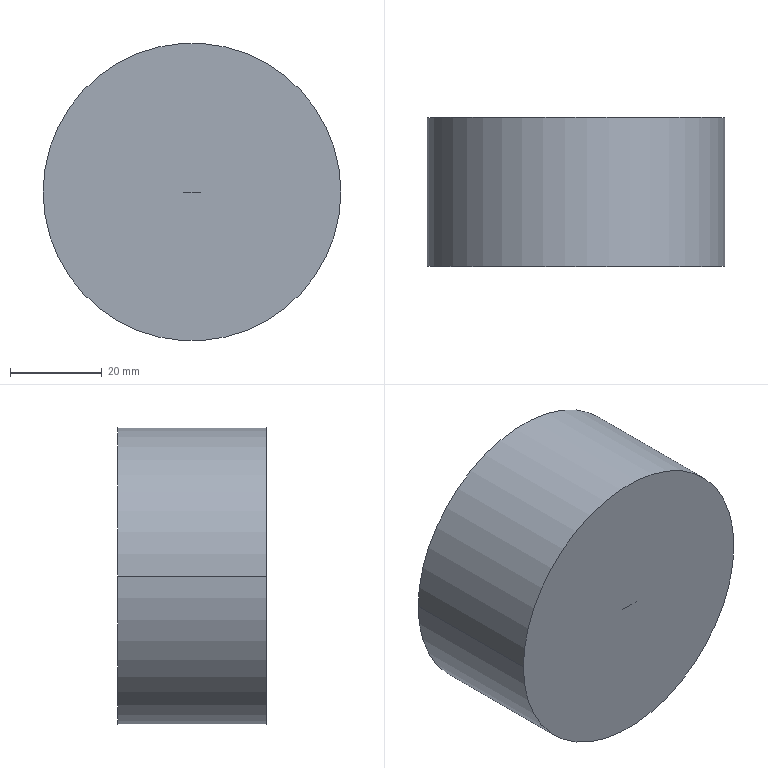Part | Creo | features DATUM PLANE 3, COORDINATE SYSTEM 1, CURVE 1, PROTRUSION 1 | 1 solid | 5 faces | box 65 x 32.5 x 65 mm | volume 35948 mm3 | cylinder 2 | sphere 2 | plane 1 | commonest cylinder face diameters 65 x2
STEP:
#1=CARTESIAN_POINT('',(0.,0.,0.));
#2=DIRECTION('',(0.,0.,1.));
#3=DIRECTION('',(1.,0.,0.));
#4=AXIS2_PLACEMENT_3D('',#1,#2,#3);
#5=CARTESIAN_POINT('',(32.5,0.,0.));
#6=VERTEX_POINT('',#5);
#7=CARTESIAN_POINT('',(-32.5,0.,0.));
#8=VERTEX_POINT('',#7);
#9=CARTESIAN_POINT('',(0.,0.,0.));
#10=DIRECTION('',(0.,-1.,0.));
#11=DIRECTION('',(1.,0.,0.));
#12=AXIS2_PLACEMENT_3D('',#9,#10,#11);
#13=CIRCLE('',#12,32.5);
#14=EDGE_CURVE('',#6,#8,#13,.T.);
#15=ORIENTED_EDGE('',*,*,#14,.F.);
#16=CARTESIAN_POINT('',(0.,0.,0.));
#17=DIRECTION('',(0.,1.,0.));
#18=DIRECTION('',(1.,0.,0.));
#19=AXIS2_PLACEMENT_3D('',#16,#17,#18);
#20=CIRCLE('',#19,32.5);
#21=EDGE_CURVE('',#6,#8,#20,.T.);
#22=ORIENTED_EDGE('',*,*,#21,.T.);
#23=EDGE_LOOP('',(#15,#22));
#24=FACE_OUTER_BOUND('',#23,.F.);
#25=CARTESIAN_POINT('',(0.,0.,0.));
#26=DIRECTION('',(0.,1.,0.));
#27=DIRECTION('',(1.,0.,0.));
#28=AXIS2_PLACEMENT_3D('',#25,#26,#27);
#29=PLANE('',#28);
#30=ADVANCED_FACE('',(#24),#29,.F.);
#31=CARTESIAN_POINT('',(32.5,32.5,0.));
#32=VERTEX_POINT('',#31);
#33=CARTESIAN_POINT('',(32.5,0.,0.));
#34=DIRECTION('',(0.,1.,0.));
#35=VECTOR('',#34,32.5);
#36=LINE('',#33,#35);
#37=EDGE_CURVE('',#6,#32,#36,.T.);
#38=ORIENTED_EDGE('',*,*,#37,.F.);
#39=ORIENTED_EDGE('',*,*,#14,.T.);
#40=CARTESIAN_POINT('',(-32.5,32.5,0.));
#41=VERTEX_POINT('',#40);
#42=CARTESIAN_POINT('',(-32.5,0.,0.));
#43=DIRECTION('',(0.,1.,0.));
#44=VECTOR('',#43,32.5);
#45=LINE('',#42,#44);
#46=EDGE_CURVE('',#8,#41,#45,.T.);
#47=ORIENTED_EDGE('',*,*,#46,.T.);
#48=CARTESIAN_POINT('',(0.,32.5,0.));
#49=DIRECTION('',(0.,-1.,0.));
#50=DIRECTION('',(1.,0.,0.));
#51=AXIS2_PLACEMENT_3D('',#48,#49,#50);
#52=CIRCLE('',#51,32.5);
#53=EDGE_CURVE('',#32,#41,#52,.T.);
#54=ORIENTED_EDGE('',*,*,#53,.F.);
#55=EDGE_LOOP('',(#38,#39,#47,#54));
#56=FACE_OUTER_BOUND('',#55,.F.);
#57=CARTESIAN_POINT('',(0.,0.,0.));
#58=DIRECTION('',(0.,1.,0.));
#59=DIRECTION('',(1.,0.,0.));
#60=AXIS2_PLACEMENT_3D('',#57,#58,#59);
#61=CYLINDRICAL_SURFACE('',#60,32.5);
#62=ADVANCED_FACE('',(#56),#61,.T.);
#63=ORIENTED_EDGE('',*,*,#37,.T.);
#64=CARTESIAN_POINT('',(0.,32.5,0.));
#65=DIRECTION('',(0.,1.,0.));
#66=DIRECTION('',(1.,0.,0.));
#67=AXIS2_PLACEMENT_3D('',#64,#65,#66);
#68=CIRCLE('',#67,32.5);
#69=EDGE_CURVE('',#32,#41,#68,.T.);
#70=ORIENTED_EDGE('',*,*,#69,.T.);
#71=ORIENTED_EDGE('',*,*,#46,.F.);
#72=ORIENTED_EDGE('',*,*,#21,.F.);
#73=EDGE_LOOP('',(#63,#70,#71,#72));
#74=FACE_OUTER_BOUND('',#73,.F.);
#75=CARTESIAN_POINT('',(0.,0.,0.));
#76=DIRECTION('',(0.,1.,0.));
#77=DIRECTION('',(1.,0.,0.));
#78=AXIS2_PLACEMENT_3D('',#75,#76,#77);
#79=CYLINDRICAL_SURFACE('',#78,32.5);
#80=ADVANCED_FACE('',(#74),#79,.T.);
#81=CARTESIAN_POINT('',(0.,0.,0.));
#82=VERTEX_POINT('',#81);
#83=CARTESIAN_POINT('',(0.,32.5,0.));
#84=DIRECTION('',(0.,0.,-1.));
#85=DIRECTION('',(1.,0.,0.));
#86=AXIS2_PLACEMENT_3D('',#83,#84,#85);
#87=CIRCLE('',#86,32.5);
#88=EDGE_CURVE('',#32,#82,#87,.T.);
#89=ORIENTED_EDGE('',*,*,#88,.T.);
#90=CARTESIAN_POINT('',(0.,32.5,0.));
#91=DIRECTION('',(0.,0.,1.));
#92=DIRECTION('',(-1.,0.,0.));
#93=AXIS2_PLACEMENT_3D('',#90,#91,#92);
#94=CIRCLE('',#93,32.5);
#95=EDGE_CURVE('',#41,#82,#94,.T.);
#96=ORIENTED_EDGE('',*,*,#95,.F.);
#97=ORIENTED_EDGE('',*,*,#69,.F.);
#98=EDGE_LOOP('',(#89,#96,#97));
#99=FACE_OUTER_BOUND('',#98,.F.);
#100=CARTESIAN_POINT('',(0.,32.5,0.));
#101=DIRECTION('',(0.,1.,0.));
#102=DIRECTION('',(1.,0.,0.));
#103=AXIS2_PLACEMENT_3D('',#100,#101,#102);
#104=SPHERICAL_SURFACE('',#103,32.5);
#105=ADVANCED_FACE('',(#99),#104,.F.);
#106=ORIENTED_EDGE('',*,*,#88,.F.);
#107=ORIENTED_EDGE('',*,*,#53,.T.);
#108=ORIENTED_EDGE('',*,*,#95,.T.);
#109=EDGE_LOOP('',(#106,#107,#108));
#110=FACE_OUTER_BOUND('',#109,.F.);
#111=CARTESIAN_POINT('',(0.,32.5,0.));
#112=DIRECTION('',(0.,1.,0.));
#113=DIRECTION('',(1.,0.,0.));
#114=AXIS2_PLACEMENT_3D('',#111,#112,#113);
#115=SPHERICAL_SURFACE('',#114,32.5);
#116=ADVANCED_FACE('',(#110),#115,.F.);
#117=CLOSED_SHELL('',(#30,#62,#80,#105,#116));
#118=MANIFOLD_SOLID_BREP('',#117);
#119=(LENGTH_UNIT()NAMED_UNIT(*)SI_UNIT(.MILLI.,.METRE.));
#120=UNCERTAINTY_MEASURE_WITH_UNIT(LENGTH_MEASURE(0.00975),#119,'','');
#121=(NAMED_UNIT(*)PLANE_ANGLE_UNIT()SI_UNIT($,.RADIAN.));
#122=PLANE_ANGLE_MEASURE_WITH_UNIT(PLANE_ANGLE_MEASURE(0.01745),#121);
#123=(CONVERSION_BASED_UNIT('DEGREE',#122)NAMED_UNIT(*)PLANE_ANGLE_UNIT());
#124=(NAMED_UNIT(*)SI_UNIT($,.STERADIAN.)SOLID_ANGLE_UNIT());
#125=(GEOMETRIC_REPRESENTATION_CONTEXT(3)GLOBAL_UNCERTAINTY_ASSIGNED_CONTEXT((#120))GLOBAL_UNIT_ASSIGNED_CONTEXT((#119,#123,#124))REPRESENTATION_CONTEXT('',''));
#126=ADVANCED_BREP_SHAPE_REPRESENTATION('',(#4,#118),#125);